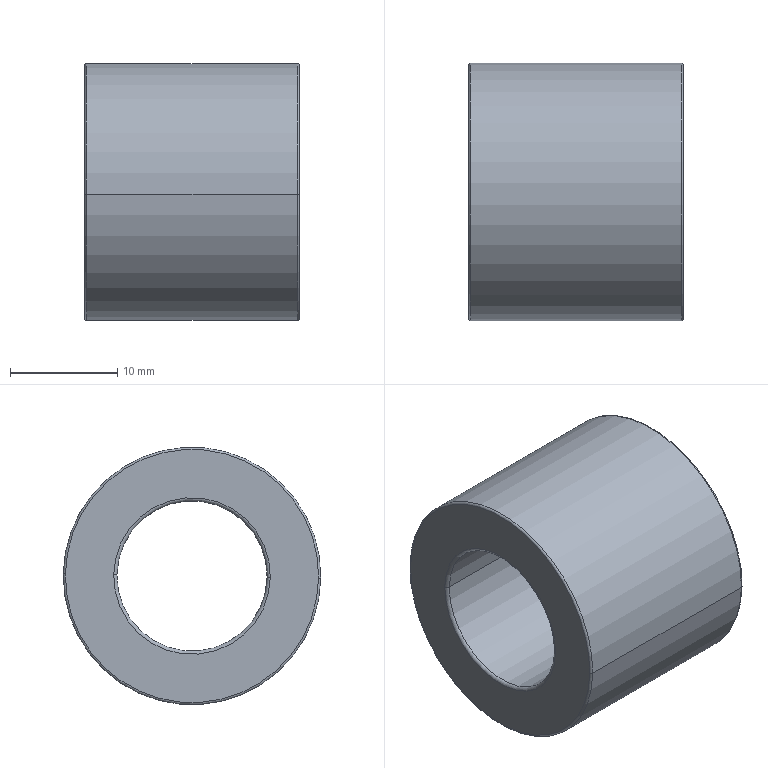Part | SolidWorks | features BaseBody 1 | 1 solid | 14 faces | box 20 x 24 x 24 mm | volume 5966 mm3 | torus 8 | cylinder 4 | plane 2 | commonest cylinder face diameters 14 x2 24 x2
STEP:
#1=CARTESIAN_POINT('',(64.5,38.799,0.1218));
#2=VERTEX_POINT('',#1);
#3=CARTESIAN_POINT('',(64.5,24.201,-0.1218));
#4=VERTEX_POINT('',#3);
#5=CARTESIAN_POINT('',(64.5,31.5,0.));
#6=DIRECTION('',(1.,0.,0.));
#7=DIRECTION('',(0.,-0.9999,-0.01668));
#8=AXIS2_PLACEMENT_3D('',#5,#6,#7);
#9=CIRCLE('',#8,7.3);
#10=EDGE_CURVE('',#2,#4,#9,.T.);
#11=ORIENTED_EDGE('',*,*,#10,.F.);
#12=CARTESIAN_POINT('',(64.8,38.499,0.1168));
#13=VERTEX_POINT('',#12);
#14=CARTESIAN_POINT('',(64.8,38.799,0.1218));
#15=DIRECTION('',(0.,-0.01668,0.9999));
#16=DIRECTION('',(0.,-0.9999,-0.01668));
#17=AXIS2_PLACEMENT_3D('',#14,#15,#16);
#18=CIRCLE('',#17,0.3);
#19=EDGE_CURVE('',#2,#13,#18,.T.);
#20=ORIENTED_EDGE('',*,*,#19,.T.);
#21=CARTESIAN_POINT('',(64.8,24.501,-0.1168));
#22=VERTEX_POINT('',#21);
#23=CARTESIAN_POINT('',(64.8,31.5,0.));
#24=DIRECTION('',(-1.,0.,0.));
#25=DIRECTION('',(0.,-0.9999,-0.01668));
#26=AXIS2_PLACEMENT_3D('',#23,#24,#25);
#27=CIRCLE('',#26,7.);
#28=EDGE_CURVE('',#22,#13,#27,.T.);
#29=ORIENTED_EDGE('',*,*,#28,.F.);
#30=CARTESIAN_POINT('',(64.8,24.201,-0.1218));
#31=DIRECTION('',(0.,0.01668,-0.9999));
#32=DIRECTION('',(0.,0.9999,0.01668));
#33=AXIS2_PLACEMENT_3D('',#30,#31,#32);
#34=CIRCLE('',#33,0.3);
#35=EDGE_CURVE('',#4,#22,#34,.T.);
#36=ORIENTED_EDGE('',*,*,#35,.F.);
#37=EDGE_LOOP('',(#11,#20,#29,#36));
#38=FACE_OUTER_BOUND('',#37,.T.);
#39=CARTESIAN_POINT('',(64.8,31.5,0.));
#40=DIRECTION('',(-1.,0.,0.));
#41=DIRECTION('',(0.,-0.9999,-0.01668));
#42=AXIS2_PLACEMENT_3D('',#39,#40,#41);
#43=TOROIDAL_SURFACE('',#42,7.3,0.3);
#44=ADVANCED_FACE('',(#38),#43,.T.);
#45=CARTESIAN_POINT('',(84.5,24.201,-0.1218));
#46=VERTEX_POINT('',#45);
#47=CARTESIAN_POINT('',(84.5,38.799,0.1218));
#48=VERTEX_POINT('',#47);
#49=CARTESIAN_POINT('',(84.5,31.5,0.));
#50=DIRECTION('',(-1.,0.,0.));
#51=DIRECTION('',(0.,0.9999,0.01668));
#52=AXIS2_PLACEMENT_3D('',#49,#50,#51);
#53=CIRCLE('',#52,7.3);
#54=EDGE_CURVE('',#46,#48,#53,.T.);
#55=ORIENTED_EDGE('',*,*,#54,.F.);
#56=CARTESIAN_POINT('',(84.2,24.501,-0.1168));
#57=VERTEX_POINT('',#56);
#58=CARTESIAN_POINT('',(84.2,24.201,-0.1218));
#59=DIRECTION('',(0.,-0.01668,0.9999));
#60=DIRECTION('',(0.,-0.9999,-0.01668));
#61=AXIS2_PLACEMENT_3D('',#58,#59,#60);
#62=CIRCLE('',#61,0.3);
#63=EDGE_CURVE('',#46,#57,#62,.T.);
#64=ORIENTED_EDGE('',*,*,#63,.T.);
#65=CARTESIAN_POINT('',(84.2,38.499,0.1168));
#66=VERTEX_POINT('',#65);
#67=CARTESIAN_POINT('',(84.2,31.5,0.));
#68=DIRECTION('',(1.,0.,0.));
#69=DIRECTION('',(0.,0.9999,0.01668));
#70=AXIS2_PLACEMENT_3D('',#67,#68,#69);
#71=CIRCLE('',#70,7.);
#72=EDGE_CURVE('',#66,#57,#71,.T.);
#73=ORIENTED_EDGE('',*,*,#72,.F.);
#74=CARTESIAN_POINT('',(84.2,38.799,0.1218));
#75=DIRECTION('',(0.,0.01668,-0.9999));
#76=DIRECTION('',(0.,0.9999,0.01668));
#77=AXIS2_PLACEMENT_3D('',#74,#75,#76);
#78=CIRCLE('',#77,0.3);
#79=EDGE_CURVE('',#48,#66,#78,.T.);
#80=ORIENTED_EDGE('',*,*,#79,.F.);
#81=EDGE_LOOP('',(#55,#64,#73,#80));
#82=FACE_OUTER_BOUND('',#81,.T.);
#83=CARTESIAN_POINT('',(84.2,31.5,0.));
#84=DIRECTION('',(1.,0.,0.));
#85=DIRECTION('',(0.,0.9999,0.01668));
#86=AXIS2_PLACEMENT_3D('',#83,#84,#85);
#87=TOROIDAL_SURFACE('',#86,7.3,0.3);
#88=ADVANCED_FACE('',(#82),#87,.T.);
#89=CARTESIAN_POINT('',(84.3,19.502,-0.2002));
#90=VERTEX_POINT('',#89);
#91=CARTESIAN_POINT('',(84.3,43.498,0.2002));
#92=VERTEX_POINT('',#91);
#93=CARTESIAN_POINT('',(84.3,31.5,0.));
#94=DIRECTION('',(-1.,0.,0.));
#95=DIRECTION('',(0.,0.9999,0.01668));
#96=AXIS2_PLACEMENT_3D('',#93,#94,#95);
#97=CIRCLE('',#96,12.);
#98=EDGE_CURVE('',#90,#92,#97,.T.);
#99=ORIENTED_EDGE('',*,*,#98,.F.);
#100=CARTESIAN_POINT('',(84.5,19.702,-0.1969));
#101=VERTEX_POINT('',#100);
#102=CARTESIAN_POINT('',(84.3,19.702,-0.1969));
#103=DIRECTION('',(0.,-0.01668,0.9999));
#104=DIRECTION('',(0.,-0.9999,-0.01668));
#105=AXIS2_PLACEMENT_3D('',#102,#103,#104);
#106=CIRCLE('',#105,0.2);
#107=EDGE_CURVE('',#90,#101,#106,.T.);
#108=ORIENTED_EDGE('',*,*,#107,.T.);
#109=CARTESIAN_POINT('',(84.5,43.298,0.1969));
#110=VERTEX_POINT('',#109);
#111=CARTESIAN_POINT('',(84.5,31.5,0.));
#112=DIRECTION('',(1.,0.,0.));
#113=DIRECTION('',(0.,0.9999,0.01668));
#114=AXIS2_PLACEMENT_3D('',#111,#112,#113);
#115=CIRCLE('',#114,11.8);
#116=EDGE_CURVE('',#110,#101,#115,.T.);
#117=ORIENTED_EDGE('',*,*,#116,.F.);
#118=CARTESIAN_POINT('',(84.3,43.298,0.1969));
#119=DIRECTION('',(0.,0.01668,-0.9999));
#120=DIRECTION('',(0.,0.9999,0.01668));
#121=AXIS2_PLACEMENT_3D('',#118,#119,#120);
#122=CIRCLE('',#121,0.2);
#123=EDGE_CURVE('',#92,#110,#122,.T.);
#124=ORIENTED_EDGE('',*,*,#123,.F.);
#125=EDGE_LOOP('',(#99,#108,#117,#124));
#126=FACE_OUTER_BOUND('',#125,.T.);
#127=CARTESIAN_POINT('',(84.3,31.5,0.));
#128=DIRECTION('',(1.,0.,0.));
#129=DIRECTION('',(0.,0.9999,0.01668));
#130=AXIS2_PLACEMENT_3D('',#127,#128,#129);
#131=TOROIDAL_SURFACE('',#130,11.8,0.2);
#132=ADVANCED_FACE('',(#126),#131,.T.);
#133=CARTESIAN_POINT('',(64.7,43.498,0.2002));
#134=VERTEX_POINT('',#133);
#135=CARTESIAN_POINT('',(64.7,19.502,-0.2002));
#136=VERTEX_POINT('',#135);
#137=CARTESIAN_POINT('',(64.7,31.5,0.));
#138=DIRECTION('',(1.,0.,0.));
#139=DIRECTION('',(0.,-0.9999,-0.01668));
#140=AXIS2_PLACEMENT_3D('',#137,#138,#139);
#141=CIRCLE('',#140,12.);
#142=EDGE_CURVE('',#134,#136,#141,.T.);
#143=ORIENTED_EDGE('',*,*,#142,.F.);
#144=CARTESIAN_POINT('',(64.5,43.298,0.1969));
#145=VERTEX_POINT('',#144);
#146=CARTESIAN_POINT('',(64.7,43.298,0.1969));
#147=DIRECTION('',(0.,-0.01668,0.9999));
#148=DIRECTION('',(0.,-0.9999,-0.01668));
#149=AXIS2_PLACEMENT_3D('',#146,#147,#148);
#150=CIRCLE('',#149,0.2);
#151=EDGE_CURVE('',#134,#145,#150,.T.);
#152=ORIENTED_EDGE('',*,*,#151,.T.);
#153=CARTESIAN_POINT('',(64.5,19.702,-0.1969));
#154=VERTEX_POINT('',#153);
#155=CARTESIAN_POINT('',(64.5,31.5,0.));
#156=DIRECTION('',(-1.,0.,0.));
#157=DIRECTION('',(0.,-0.9999,-0.01668));
#158=AXIS2_PLACEMENT_3D('',#155,#156,#157);
#159=CIRCLE('',#158,11.8);
#160=EDGE_CURVE('',#154,#145,#159,.T.);
#161=ORIENTED_EDGE('',*,*,#160,.F.);
#162=CARTESIAN_POINT('',(64.7,19.702,-0.1969));
#163=DIRECTION('',(0.,0.01668,-0.9999));
#164=DIRECTION('',(0.,0.9999,0.01668));
#165=AXIS2_PLACEMENT_3D('',#162,#163,#164);
#166=CIRCLE('',#165,0.2);
#167=EDGE_CURVE('',#136,#154,#166,.T.);
#168=ORIENTED_EDGE('',*,*,#167,.F.);
#169=EDGE_LOOP('',(#143,#152,#161,#168));
#170=FACE_OUTER_BOUND('',#169,.T.);
#171=CARTESIAN_POINT('',(64.7,31.5,0.));
#172=DIRECTION('',(-1.,0.,0.));
#173=DIRECTION('',(0.,-0.9999,-0.01668));
#174=AXIS2_PLACEMENT_3D('',#171,#172,#173);
#175=TOROIDAL_SURFACE('',#174,11.8,0.2);
#176=ADVANCED_FACE('',(#170),#175,.T.);
#177=ORIENTED_EDGE('',*,*,#142,.T.);
#178=CARTESIAN_POINT('',(84.5,19.502,-0.2002));
#179=DIRECTION('',(1.,0.,0.));
#180=VECTOR('',#179,1000.);
#181=LINE('',#178,#180);
#182=EDGE_CURVE('',#136,#90,#181,.T.);
#183=ORIENTED_EDGE('',*,*,#182,.T.);
#184=ORIENTED_EDGE('',*,*,#98,.T.);
#185=CARTESIAN_POINT('',(84.5,43.498,0.2002));
#186=DIRECTION('',(1.,0.,0.));
#187=VECTOR('',#186,1000.);
#188=LINE('',#185,#187);
#189=EDGE_CURVE('',#134,#92,#188,.T.);
#190=ORIENTED_EDGE('',*,*,#189,.F.);
#191=EDGE_LOOP('',(#177,#183,#184,#190));
#192=FACE_OUTER_BOUND('',#191,.T.);
#193=CARTESIAN_POINT('',(84.5,31.5,0.));
#194=DIRECTION('',(1.,0.,0.));
#195=DIRECTION('',(0.,0.9999,0.01668));
#196=AXIS2_PLACEMENT_3D('',#193,#194,#195);
#197=CYLINDRICAL_SURFACE('',#196,12.);
#198=ADVANCED_FACE('',(#192),#197,.T.);
#199=CARTESIAN_POINT('',(64.8,31.5,0.));
#200=DIRECTION('',(-1.,0.,0.));
#201=DIRECTION('',(0.,-0.9999,-0.01668));
#202=AXIS2_PLACEMENT_3D('',#199,#200,#201);
#203=CIRCLE('',#202,7.);
#204=EDGE_CURVE('',#13,#22,#203,.T.);
#205=ORIENTED_EDGE('',*,*,#204,.T.);
#206=CARTESIAN_POINT('',(84.5,24.501,-0.1168));
#207=DIRECTION('',(1.,0.,0.));
#208=VECTOR('',#207,1000.);
#209=LINE('',#206,#208);
#210=EDGE_CURVE('',#22,#57,#209,.T.);
#211=ORIENTED_EDGE('',*,*,#210,.T.);
#212=CARTESIAN_POINT('',(84.2,31.5,0.));
#213=DIRECTION('',(1.,0.,0.));
#214=DIRECTION('',(0.,0.9999,0.01668));
#215=AXIS2_PLACEMENT_3D('',#212,#213,#214);
#216=CIRCLE('',#215,7.);
#217=EDGE_CURVE('',#57,#66,#216,.T.);
#218=ORIENTED_EDGE('',*,*,#217,.T.);
#219=CARTESIAN_POINT('',(84.5,38.499,0.1168));
#220=DIRECTION('',(1.,0.,0.));
#221=VECTOR('',#220,1000.);
#222=LINE('',#219,#221);
#223=EDGE_CURVE('',#13,#66,#222,.T.);
#224=ORIENTED_EDGE('',*,*,#223,.F.);
#225=EDGE_LOOP('',(#205,#211,#218,#224));
#226=FACE_OUTER_BOUND('',#225,.T.);
#227=CARTESIAN_POINT('',(84.5,31.5,0.));
#228=DIRECTION('',(1.,0.,0.));
#229=DIRECTION('',(0.,0.9999,0.01668));
#230=AXIS2_PLACEMENT_3D('',#227,#228,#229);
#231=CYLINDRICAL_SURFACE('',#230,7.);
#232=ADVANCED_FACE('',(#226),#231,.F.);
#233=ORIENTED_EDGE('',*,*,#210,.F.);
#234=ORIENTED_EDGE('',*,*,#28,.T.);
#235=ORIENTED_EDGE('',*,*,#223,.T.);
#236=ORIENTED_EDGE('',*,*,#72,.T.);
#237=EDGE_LOOP('',(#233,#234,#235,#236));
#238=FACE_OUTER_BOUND('',#237,.T.);
#239=CARTESIAN_POINT('',(84.5,31.5,0.));
#240=DIRECTION('',(1.,0.,0.));
#241=DIRECTION('',(0.,0.9999,0.01668));
#242=AXIS2_PLACEMENT_3D('',#239,#240,#241);
#243=CYLINDRICAL_SURFACE('',#242,7.);
#244=ADVANCED_FACE('',(#238),#243,.F.);
#245=CARTESIAN_POINT('',(64.5,31.5,0.));
#246=DIRECTION('',(1.,0.,0.));
#247=DIRECTION('',(0.,-0.9999,-0.01668));
#248=AXIS2_PLACEMENT_3D('',#245,#246,#247);
#249=CIRCLE('',#248,7.3);
#250=EDGE_CURVE('',#4,#2,#249,.T.);
#251=ORIENTED_EDGE('',*,*,#250,.T.);
#252=ORIENTED_EDGE('',*,*,#10,.T.);
#253=EDGE_LOOP('',(#251,#252));
#254=FACE_BOUND('',#253,.T.);
#255=ORIENTED_EDGE('',*,*,#160,.T.);
#256=CARTESIAN_POINT('',(64.5,31.5,0.));
#257=DIRECTION('',(-1.,0.,0.));
#258=DIRECTION('',(0.,-0.9999,-0.01668));
#259=AXIS2_PLACEMENT_3D('',#256,#257,#258);
#260=CIRCLE('',#259,11.8);
#261=EDGE_CURVE('',#145,#154,#260,.T.);
#262=ORIENTED_EDGE('',*,*,#261,.T.);
#263=EDGE_LOOP('',(#255,#262));
#264=FACE_OUTER_BOUND('',#263,.T.);
#265=CARTESIAN_POINT('',(64.5,31.383,6.999));
#266=DIRECTION('',(-1.,0.,0.));
#267=DIRECTION('',(0.,-0.9999,-0.01668));
#268=AXIS2_PLACEMENT_3D('',#265,#266,#267);
#269=PLANE('',#268);
#270=ADVANCED_FACE('',(#254,#264),#269,.T.);
#271=ORIENTED_EDGE('',*,*,#182,.F.);
#272=CARTESIAN_POINT('',(64.7,31.5,0.));
#273=DIRECTION('',(1.,0.,0.));
#274=DIRECTION('',(0.,-0.9999,-0.01668));
#275=AXIS2_PLACEMENT_3D('',#272,#273,#274);
#276=CIRCLE('',#275,12.);
#277=EDGE_CURVE('',#136,#134,#276,.T.);
#278=ORIENTED_EDGE('',*,*,#277,.T.);
#279=ORIENTED_EDGE('',*,*,#189,.T.);
#280=CARTESIAN_POINT('',(84.3,31.5,0.));
#281=DIRECTION('',(-1.,0.,0.));
#282=DIRECTION('',(0.,0.9999,0.01668));
#283=AXIS2_PLACEMENT_3D('',#280,#281,#282);
#284=CIRCLE('',#283,12.);
#285=EDGE_CURVE('',#92,#90,#284,.T.);
#286=ORIENTED_EDGE('',*,*,#285,.T.);
#287=EDGE_LOOP('',(#271,#278,#279,#286));
#288=FACE_OUTER_BOUND('',#287,.T.);
#289=CARTESIAN_POINT('',(84.5,31.5,0.));
#290=DIRECTION('',(1.,0.,0.));
#291=DIRECTION('',(0.,0.9999,0.01668));
#292=AXIS2_PLACEMENT_3D('',#289,#290,#291);
#293=CYLINDRICAL_SURFACE('',#292,12.);
#294=ADVANCED_FACE('',(#288),#293,.T.);
#295=CARTESIAN_POINT('',(84.5,31.5,0.));
#296=DIRECTION('',(-1.,0.,0.));
#297=DIRECTION('',(0.,0.9999,0.01668));
#298=AXIS2_PLACEMENT_3D('',#295,#296,#297);
#299=CIRCLE('',#298,7.3);
#300=EDGE_CURVE('',#48,#46,#299,.T.);
#301=ORIENTED_EDGE('',*,*,#300,.T.);
#302=ORIENTED_EDGE('',*,*,#54,.T.);
#303=EDGE_LOOP('',(#301,#302));
#304=FACE_BOUND('',#303,.T.);
#305=ORIENTED_EDGE('',*,*,#116,.T.);
#306=CARTESIAN_POINT('',(84.5,31.5,0.));
#307=DIRECTION('',(1.,0.,0.));
#308=DIRECTION('',(0.,0.9999,0.01668));
#309=AXIS2_PLACEMENT_3D('',#306,#307,#308);
#310=CIRCLE('',#309,11.8);
#311=EDGE_CURVE('',#101,#110,#310,.T.);
#312=ORIENTED_EDGE('',*,*,#311,.T.);
#313=EDGE_LOOP('',(#305,#312));
#314=FACE_OUTER_BOUND('',#313,.T.);
#315=CARTESIAN_POINT('',(84.5,31.3,11.998));
#316=DIRECTION('',(1.,0.,0.));
#317=DIRECTION('',(0.,0.9999,0.01668));
#318=AXIS2_PLACEMENT_3D('',#315,#316,#317);
#319=PLANE('',#318);
#320=ADVANCED_FACE('',(#304,#314),#319,.T.);
#321=ORIENTED_EDGE('',*,*,#151,.F.);
#322=ORIENTED_EDGE('',*,*,#277,.F.);
#323=ORIENTED_EDGE('',*,*,#167,.T.);
#324=ORIENTED_EDGE('',*,*,#261,.F.);
#325=EDGE_LOOP('',(#321,#322,#323,#324));
#326=FACE_OUTER_BOUND('',#325,.T.);
#327=CARTESIAN_POINT('',(64.7,31.5,0.));
#328=DIRECTION('',(-1.,0.,0.));
#329=DIRECTION('',(0.,-0.9999,-0.01668));
#330=AXIS2_PLACEMENT_3D('',#327,#328,#329);
#331=TOROIDAL_SURFACE('',#330,11.8,0.2);
#332=ADVANCED_FACE('',(#326),#331,.T.);
#333=ORIENTED_EDGE('',*,*,#107,.F.);
#334=ORIENTED_EDGE('',*,*,#285,.F.);
#335=ORIENTED_EDGE('',*,*,#123,.T.);
#336=ORIENTED_EDGE('',*,*,#311,.F.);
#337=EDGE_LOOP('',(#333,#334,#335,#336));
#338=FACE_OUTER_BOUND('',#337,.T.);
#339=CARTESIAN_POINT('',(84.3,31.5,0.));
#340=DIRECTION('',(1.,0.,0.));
#341=DIRECTION('',(0.,0.9999,0.01668));
#342=AXIS2_PLACEMENT_3D('',#339,#340,#341);
#343=TOROIDAL_SURFACE('',#342,11.8,0.2);
#344=ADVANCED_FACE('',(#338),#343,.T.);
#345=ORIENTED_EDGE('',*,*,#63,.F.);
#346=ORIENTED_EDGE('',*,*,#300,.F.);
#347=ORIENTED_EDGE('',*,*,#79,.T.);
#348=ORIENTED_EDGE('',*,*,#217,.F.);
#349=EDGE_LOOP('',(#345,#346,#347,#348));
#350=FACE_OUTER_BOUND('',#349,.T.);
#351=CARTESIAN_POINT('',(84.2,31.5,0.));
#352=DIRECTION('',(1.,0.,0.));
#353=DIRECTION('',(0.,0.9999,0.01668));
#354=AXIS2_PLACEMENT_3D('',#351,#352,#353);
#355=TOROIDAL_SURFACE('',#354,7.3,0.3);
#356=ADVANCED_FACE('',(#350),#355,.T.);
#357=ORIENTED_EDGE('',*,*,#19,.F.);
#358=ORIENTED_EDGE('',*,*,#250,.F.);
#359=ORIENTED_EDGE('',*,*,#35,.T.);
#360=ORIENTED_EDGE('',*,*,#204,.F.);
#361=EDGE_LOOP('',(#357,#358,#359,#360));
#362=FACE_OUTER_BOUND('',#361,.T.);
#363=CARTESIAN_POINT('',(64.8,31.5,0.));
#364=DIRECTION('',(-1.,0.,0.));
#365=DIRECTION('',(0.,-0.9999,-0.01668));
#366=AXIS2_PLACEMENT_3D('',#363,#364,#365);
#367=TOROIDAL_SURFACE('',#366,7.3,0.3);
#368=ADVANCED_FACE('',(#362),#367,.T.);
#369=CLOSED_SHELL('',(#44,#88,#132,#176,#198,#232,#244,#270,#294,#320,#332,#344,#356,#368));
#370=MANIFOLD_SOLID_BREP('',#369);
#371=CARTESIAN_POINT('',(0.,0.,0.));
#372=DIRECTION('',(0.,0.,1.));
#373=DIRECTION('',(1.,0.,0.));
#374=AXIS2_PLACEMENT_3D('',#371,#372,#373);
#375=(LENGTH_UNIT()NAMED_UNIT(*)SI_UNIT(.MILLI.,.METRE.));
#376=UNCERTAINTY_MEASURE_WITH_UNIT(LENGTH_MEASURE(0.00001),#375,'','');
#377=(NAMED_UNIT(*)PLANE_ANGLE_UNIT()SI_UNIT($,.RADIAN.));
#378=(NAMED_UNIT(*)SI_UNIT($,.STERADIAN.)SOLID_ANGLE_UNIT());
#379=(GEOMETRIC_REPRESENTATION_CONTEXT(3)GLOBAL_UNCERTAINTY_ASSIGNED_CONTEXT((#376))GLOBAL_UNIT_ASSIGNED_CONTEXT((#375,#377,#378))REPRESENTATION_CONTEXT('',''));
#380=ADVANCED_BREP_SHAPE_REPRESENTATION('',(#370,#374),#379);